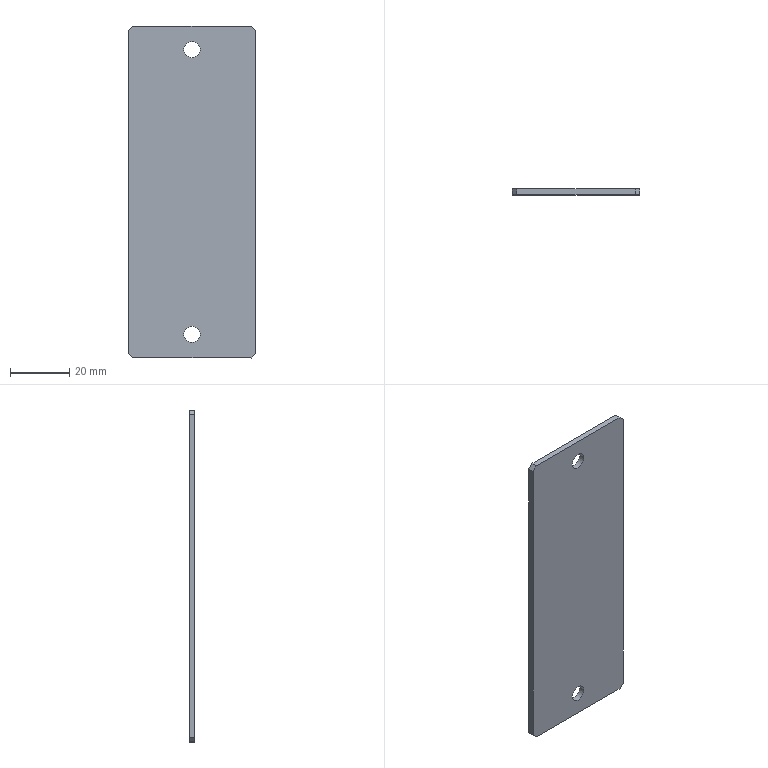Part | NX | 1 solid | 12 faces | box 43 x 2 x 112 mm | volume 9528 mm3 | plane 10 | cylinder 2 | commonest cylinder face diameters 5.5 x2
STEP:
#1=CARTESIAN_POINT('',(21.5,2.,54.5));
#2=VERTEX_POINT('',#1);
#3=CARTESIAN_POINT('',(21.5,2.,-54.5));
#4=VERTEX_POINT('',#3);
#5=CARTESIAN_POINT('',(21.5,2.,-56.));
#6=DIRECTION('',(0.,0.,-1.));
#7=VECTOR('',#6,1000.);
#8=LINE('',#5,#7);
#9=EDGE_CURVE('',#2,#4,#8,.T.);
#10=ORIENTED_EDGE('',*,*,#9,.F.);
#11=CARTESIAN_POINT('',(21.5,0.,54.5));
#12=VERTEX_POINT('',#11);
#13=CARTESIAN_POINT('',(21.5,2.,54.5));
#14=DIRECTION('',(0.,-1.,0.));
#15=VECTOR('',#14,1000.);
#16=LINE('',#13,#15);
#17=EDGE_CURVE('',#2,#12,#16,.T.);
#18=ORIENTED_EDGE('',*,*,#17,.T.);
#19=CARTESIAN_POINT('',(21.5,0.,-54.5));
#20=VERTEX_POINT('',#19);
#21=CARTESIAN_POINT('',(21.5,0.,-56.));
#22=DIRECTION('',(0.,0.,-1.));
#23=VECTOR('',#22,1000.);
#24=LINE('',#21,#23);
#25=EDGE_CURVE('',#12,#20,#24,.T.);
#26=ORIENTED_EDGE('',*,*,#25,.T.);
#27=CARTESIAN_POINT('',(21.5,2.,-54.5));
#28=DIRECTION('',(0.,1.,0.));
#29=VECTOR('',#28,1000.);
#30=LINE('',#27,#29);
#31=EDGE_CURVE('',#20,#4,#30,.T.);
#32=ORIENTED_EDGE('',*,*,#31,.T.);
#33=EDGE_LOOP('',(#10,#18,#26,#32));
#34=FACE_BOUND('',#33,.T.);
#35=CARTESIAN_POINT('',(21.5,2.,-56.));
#36=DIRECTION('',(-1.,0.,0.));
#37=DIRECTION('',(0.,0.,1.));
#38=AXIS2_PLACEMENT_3D('',#35,#36,#37);
#39=PLANE('',#38);
#40=ADVANCED_FACE('',(#34),#39,.F.);
#41=CARTESIAN_POINT('',(20.,2.,-56.));
#42=VERTEX_POINT('',#41);
#43=CARTESIAN_POINT('',(-20.,2.,-56.));
#44=VERTEX_POINT('',#43);
#45=CARTESIAN_POINT('',(-21.5,2.,-56.));
#46=DIRECTION('',(-1.,0.,0.));
#47=VECTOR('',#46,1000.);
#48=LINE('',#45,#47);
#49=EDGE_CURVE('',#42,#44,#48,.T.);
#50=ORIENTED_EDGE('',*,*,#49,.F.);
#51=CARTESIAN_POINT('',(20.,0.,-56.));
#52=VERTEX_POINT('',#51);
#53=CARTESIAN_POINT('',(20.,2.,-56.));
#54=DIRECTION('',(0.,-1.,0.));
#55=VECTOR('',#54,1000.);
#56=LINE('',#53,#55);
#57=EDGE_CURVE('',#42,#52,#56,.T.);
#58=ORIENTED_EDGE('',*,*,#57,.T.);
#59=CARTESIAN_POINT('',(-20.,0.,-56.));
#60=VERTEX_POINT('',#59);
#61=CARTESIAN_POINT('',(-21.5,0.,-56.));
#62=DIRECTION('',(-1.,0.,0.));
#63=VECTOR('',#62,1000.);
#64=LINE('',#61,#63);
#65=EDGE_CURVE('',#52,#60,#64,.T.);
#66=ORIENTED_EDGE('',*,*,#65,.T.);
#67=CARTESIAN_POINT('',(-20.,2.,-56.));
#68=DIRECTION('',(0.,1.,0.));
#69=VECTOR('',#68,1000.);
#70=LINE('',#67,#69);
#71=EDGE_CURVE('',#60,#44,#70,.T.);
#72=ORIENTED_EDGE('',*,*,#71,.T.);
#73=EDGE_LOOP('',(#50,#58,#66,#72));
#74=FACE_BOUND('',#73,.T.);
#75=CARTESIAN_POINT('',(-21.5,2.,-56.));
#76=DIRECTION('',(0.,0.,1.));
#77=DIRECTION('',(1.,0.,0.));
#78=AXIS2_PLACEMENT_3D('',#75,#76,#77);
#79=PLANE('',#78);
#80=ADVANCED_FACE('',(#74),#79,.F.);
#81=CARTESIAN_POINT('',(-21.5,0.,-54.5));
#82=VERTEX_POINT('',#81);
#83=CARTESIAN_POINT('',(-21.5,0.,54.5));
#84=VERTEX_POINT('',#83);
#85=CARTESIAN_POINT('',(-21.5,0.,-56.));
#86=DIRECTION('',(0.,0.,1.));
#87=VECTOR('',#86,1000.);
#88=LINE('',#85,#87);
#89=EDGE_CURVE('',#82,#84,#88,.T.);
#90=ORIENTED_EDGE('',*,*,#89,.T.);
#91=CARTESIAN_POINT('',(-21.5,2.,54.5));
#92=VERTEX_POINT('',#91);
#93=CARTESIAN_POINT('',(-21.5,2.,54.5));
#94=DIRECTION('',(0.,1.,0.));
#95=VECTOR('',#94,1000.);
#96=LINE('',#93,#95);
#97=EDGE_CURVE('',#84,#92,#96,.T.);
#98=ORIENTED_EDGE('',*,*,#97,.T.);
#99=CARTESIAN_POINT('',(-21.5,2.,-54.5));
#100=VERTEX_POINT('',#99);
#101=CARTESIAN_POINT('',(-21.5,2.,-56.));
#102=DIRECTION('',(0.,0.,1.));
#103=VECTOR('',#102,1000.);
#104=LINE('',#101,#103);
#105=EDGE_CURVE('',#100,#92,#104,.T.);
#106=ORIENTED_EDGE('',*,*,#105,.F.);
#107=CARTESIAN_POINT('',(-21.5,2.,-54.5));
#108=DIRECTION('',(0.,-1.,0.));
#109=VECTOR('',#108,1000.);
#110=LINE('',#107,#109);
#111=EDGE_CURVE('',#100,#82,#110,.T.);
#112=ORIENTED_EDGE('',*,*,#111,.T.);
#113=EDGE_LOOP('',(#90,#98,#106,#112));
#114=FACE_BOUND('',#113,.T.);
#115=CARTESIAN_POINT('',(-21.5,2.,-56.));
#116=DIRECTION('',(1.,0.,0.));
#117=DIRECTION('',(0.,0.,-1.));
#118=AXIS2_PLACEMENT_3D('',#115,#116,#117);
#119=PLANE('',#118);
#120=ADVANCED_FACE('',(#114),#119,.F.);
#121=CARTESIAN_POINT('',(-20.,2.,56.));
#122=VERTEX_POINT('',#121);
#123=CARTESIAN_POINT('',(20.,2.,56.));
#124=VERTEX_POINT('',#123);
#125=CARTESIAN_POINT('',(-21.5,2.,56.));
#126=DIRECTION('',(1.,0.,0.));
#127=VECTOR('',#126,1000.);
#128=LINE('',#125,#127);
#129=EDGE_CURVE('',#122,#124,#128,.T.);
#130=ORIENTED_EDGE('',*,*,#129,.F.);
#131=CARTESIAN_POINT('',(-20.,0.,56.));
#132=VERTEX_POINT('',#131);
#133=CARTESIAN_POINT('',(-20.,2.,56.));
#134=DIRECTION('',(0.,-1.,0.));
#135=VECTOR('',#134,1000.);
#136=LINE('',#133,#135);
#137=EDGE_CURVE('',#122,#132,#136,.T.);
#138=ORIENTED_EDGE('',*,*,#137,.T.);
#139=CARTESIAN_POINT('',(20.,0.,56.));
#140=VERTEX_POINT('',#139);
#141=CARTESIAN_POINT('',(-21.5,0.,56.));
#142=DIRECTION('',(1.,0.,0.));
#143=VECTOR('',#142,1000.);
#144=LINE('',#141,#143);
#145=EDGE_CURVE('',#132,#140,#144,.T.);
#146=ORIENTED_EDGE('',*,*,#145,.T.);
#147=CARTESIAN_POINT('',(20.,2.,56.));
#148=DIRECTION('',(0.,1.,0.));
#149=VECTOR('',#148,1000.);
#150=LINE('',#147,#149);
#151=EDGE_CURVE('',#140,#124,#150,.T.);
#152=ORIENTED_EDGE('',*,*,#151,.T.);
#153=EDGE_LOOP('',(#130,#138,#146,#152));
#154=FACE_BOUND('',#153,.T.);
#155=CARTESIAN_POINT('',(-21.5,2.,56.));
#156=DIRECTION('',(0.,0.,-1.));
#157=DIRECTION('',(-1.,0.,0.));
#158=AXIS2_PLACEMENT_3D('',#155,#156,#157);
#159=PLANE('',#158);
#160=ADVANCED_FACE('',(#154),#159,.F.);
#161=CARTESIAN_POINT('',(0.,2.,50.75));
#162=VERTEX_POINT('',#161);
#163=CARTESIAN_POINT('',(0.,2.,48.));
#164=DIRECTION('',(0.,1.,0.));
#165=DIRECTION('',(0.,0.,1.));
#166=AXIS2_PLACEMENT_3D('',#163,#164,#165);
#167=CIRCLE('',#166,2.75);
#168=EDGE_CURVE('',#162,#162,#167,.T.);
#169=ORIENTED_EDGE('',*,*,#168,.F.);
#170=EDGE_LOOP('',(#169));
#171=FACE_BOUND('',#170,.T.);
#172=CARTESIAN_POINT('',(0.,2.,-45.25));
#173=VERTEX_POINT('',#172);
#174=CARTESIAN_POINT('',(0.,2.,-48.));
#175=DIRECTION('',(0.,1.,0.));
#176=DIRECTION('',(0.,0.,1.));
#177=AXIS2_PLACEMENT_3D('',#174,#175,#176);
#178=CIRCLE('',#177,2.75);
#179=EDGE_CURVE('',#173,#173,#178,.T.);
#180=ORIENTED_EDGE('',*,*,#179,.F.);
#181=EDGE_LOOP('',(#180));
#182=FACE_BOUND('',#181,.T.);
#183=ORIENTED_EDGE('',*,*,#105,.T.);
#184=CARTESIAN_POINT('',(-38.,2.,38.));
#185=DIRECTION('',(-0.7071,0.,-0.7071));
#186=VECTOR('',#185,1000.);
#187=LINE('',#184,#186);
#188=EDGE_CURVE('',#92,#122,#187,.F.);
#189=ORIENTED_EDGE('',*,*,#188,.T.);
#190=ORIENTED_EDGE('',*,*,#129,.T.);
#191=CARTESIAN_POINT('',(38.,2.,38.));
#192=DIRECTION('',(-0.7071,0.,0.7071));
#193=VECTOR('',#192,1000.);
#194=LINE('',#191,#193);
#195=EDGE_CURVE('',#124,#2,#194,.F.);
#196=ORIENTED_EDGE('',*,*,#195,.T.);
#197=ORIENTED_EDGE('',*,*,#9,.T.);
#198=CARTESIAN_POINT('',(38.,2.,-38.));
#199=DIRECTION('',(0.7071,0.,0.7071));
#200=VECTOR('',#199,1000.);
#201=LINE('',#198,#200);
#202=EDGE_CURVE('',#4,#42,#201,.F.);
#203=ORIENTED_EDGE('',*,*,#202,.T.);
#204=ORIENTED_EDGE('',*,*,#49,.T.);
#205=CARTESIAN_POINT('',(-38.,2.,-38.));
#206=DIRECTION('',(0.7071,0.,-0.7071));
#207=VECTOR('',#206,1000.);
#208=LINE('',#205,#207);
#209=EDGE_CURVE('',#44,#100,#208,.F.);
#210=ORIENTED_EDGE('',*,*,#209,.T.);
#211=EDGE_LOOP('',(#183,#189,#190,#196,#197,#203,#204,#210));
#212=FACE_BOUND('',#211,.T.);
#213=CARTESIAN_POINT('',(0.,2.,0.));
#214=DIRECTION('',(0.,1.,0.));
#215=DIRECTION('',(0.,0.,1.));
#216=AXIS2_PLACEMENT_3D('',#213,#214,#215);
#217=PLANE('',#216);
#218=ADVANCED_FACE('',(#171,#182,#212),#217,.T.);
#219=CARTESIAN_POINT('',(0.,0.,50.75));
#220=VERTEX_POINT('',#219);
#221=CARTESIAN_POINT('',(0.,0.,48.));
#222=DIRECTION('',(0.,1.,0.));
#223=DIRECTION('',(0.,0.,1.));
#224=AXIS2_PLACEMENT_3D('',#221,#222,#223);
#225=CIRCLE('',#224,2.75);
#226=EDGE_CURVE('',#220,#220,#225,.T.);
#227=ORIENTED_EDGE('',*,*,#226,.T.);
#228=EDGE_LOOP('',(#227));
#229=FACE_BOUND('',#228,.T.);
#230=CARTESIAN_POINT('',(0.,0.,-45.25));
#231=VERTEX_POINT('',#230);
#232=CARTESIAN_POINT('',(0.,0.,-48.));
#233=DIRECTION('',(0.,1.,0.));
#234=DIRECTION('',(0.,0.,1.));
#235=AXIS2_PLACEMENT_3D('',#232,#233,#234);
#236=CIRCLE('',#235,2.75);
#237=EDGE_CURVE('',#231,#231,#236,.T.);
#238=ORIENTED_EDGE('',*,*,#237,.T.);
#239=EDGE_LOOP('',(#238));
#240=FACE_BOUND('',#239,.T.);
#241=ORIENTED_EDGE('',*,*,#145,.F.);
#242=CARTESIAN_POINT('',(-20.,0.,56.));
#243=DIRECTION('',(0.7071,0.,0.7071));
#244=VECTOR('',#243,1000.);
#245=LINE('',#242,#244);
#246=EDGE_CURVE('',#132,#84,#245,.F.);
#247=ORIENTED_EDGE('',*,*,#246,.T.);
#248=ORIENTED_EDGE('',*,*,#89,.F.);
#249=CARTESIAN_POINT('',(-21.5,0.,-54.5));
#250=DIRECTION('',(-0.7071,0.,0.7071));
#251=VECTOR('',#250,1000.);
#252=LINE('',#249,#251);
#253=EDGE_CURVE('',#82,#60,#252,.F.);
#254=ORIENTED_EDGE('',*,*,#253,.T.);
#255=ORIENTED_EDGE('',*,*,#65,.F.);
#256=CARTESIAN_POINT('',(20.,0.,-56.));
#257=DIRECTION('',(-0.7071,0.,-0.7071));
#258=VECTOR('',#257,1000.);
#259=LINE('',#256,#258);
#260=EDGE_CURVE('',#52,#20,#259,.F.);
#261=ORIENTED_EDGE('',*,*,#260,.T.);
#262=ORIENTED_EDGE('',*,*,#25,.F.);
#263=CARTESIAN_POINT('',(21.5,0.,54.5));
#264=DIRECTION('',(0.7071,0.,-0.7071));
#265=VECTOR('',#264,1000.);
#266=LINE('',#263,#265);
#267=EDGE_CURVE('',#12,#140,#266,.F.);
#268=ORIENTED_EDGE('',*,*,#267,.T.);
#269=EDGE_LOOP('',(#241,#247,#248,#254,#255,#261,#262,#268));
#270=FACE_BOUND('',#269,.T.);
#271=CARTESIAN_POINT('',(0.,0.,0.));
#272=DIRECTION('',(0.,1.,0.));
#273=DIRECTION('',(0.,0.,1.));
#274=AXIS2_PLACEMENT_3D('',#271,#272,#273);
#275=PLANE('',#274);
#276=ADVANCED_FACE('',(#229,#240,#270),#275,.F.);
#277=ORIENTED_EDGE('',*,*,#237,.F.);
#278=EDGE_LOOP('',(#277));
#279=FACE_BOUND('',#278,.T.);
#280=ORIENTED_EDGE('',*,*,#179,.T.);
#281=EDGE_LOOP('',(#280));
#282=FACE_BOUND('',#281,.T.);
#283=CARTESIAN_POINT('',(0.,2.,-48.));
#284=DIRECTION('',(0.,1.,0.));
#285=DIRECTION('',(0.,0.,1.));
#286=AXIS2_PLACEMENT_3D('',#283,#284,#285);
#287=CYLINDRICAL_SURFACE('',#286,2.75);
#288=ADVANCED_FACE('',(#279,#282),#287,.F.);
#289=ORIENTED_EDGE('',*,*,#226,.F.);
#290=EDGE_LOOP('',(#289));
#291=FACE_BOUND('',#290,.T.);
#292=ORIENTED_EDGE('',*,*,#168,.T.);
#293=EDGE_LOOP('',(#292));
#294=FACE_BOUND('',#293,.T.);
#295=CARTESIAN_POINT('',(0.,2.,48.));
#296=DIRECTION('',(0.,1.,0.));
#297=DIRECTION('',(0.,0.,1.));
#298=AXIS2_PLACEMENT_3D('',#295,#296,#297);
#299=CYLINDRICAL_SURFACE('',#298,2.75);
#300=ADVANCED_FACE('',(#291,#294),#299,.F.);
#301=ORIENTED_EDGE('',*,*,#188,.F.);
#302=ORIENTED_EDGE('',*,*,#97,.F.);
#303=ORIENTED_EDGE('',*,*,#246,.F.);
#304=ORIENTED_EDGE('',*,*,#137,.F.);
#305=EDGE_LOOP('',(#301,#302,#303,#304));
#306=FACE_BOUND('',#305,.T.);
#307=CARTESIAN_POINT('',(-20.,2.,56.));
#308=DIRECTION('',(0.7071,0.,-0.7071));
#309=DIRECTION('',(0.,-1.,0.));
#310=AXIS2_PLACEMENT_3D('',#307,#308,#309);
#311=PLANE('',#310);
#312=ADVANCED_FACE('',(#306),#311,.F.);
#313=ORIENTED_EDGE('',*,*,#195,.F.);
#314=ORIENTED_EDGE('',*,*,#151,.F.);
#315=ORIENTED_EDGE('',*,*,#267,.F.);
#316=ORIENTED_EDGE('',*,*,#17,.F.);
#317=EDGE_LOOP('',(#313,#314,#315,#316));
#318=FACE_BOUND('',#317,.T.);
#319=CARTESIAN_POINT('',(21.5,2.,54.5));
#320=DIRECTION('',(-0.7071,0.,-0.7071));
#321=DIRECTION('',(0.,-1.,0.));
#322=AXIS2_PLACEMENT_3D('',#319,#320,#321);
#323=PLANE('',#322);
#324=ADVANCED_FACE('',(#318),#323,.F.);
#325=ORIENTED_EDGE('',*,*,#202,.F.);
#326=ORIENTED_EDGE('',*,*,#31,.F.);
#327=ORIENTED_EDGE('',*,*,#260,.F.);
#328=ORIENTED_EDGE('',*,*,#57,.F.);
#329=EDGE_LOOP('',(#325,#326,#327,#328));
#330=FACE_BOUND('',#329,.T.);
#331=CARTESIAN_POINT('',(20.,2.,-56.));
#332=DIRECTION('',(-0.7071,0.,0.7071));
#333=DIRECTION('',(0.,-1.,0.));
#334=AXIS2_PLACEMENT_3D('',#331,#332,#333);
#335=PLANE('',#334);
#336=ADVANCED_FACE('',(#330),#335,.F.);
#337=ORIENTED_EDGE('',*,*,#209,.F.);
#338=ORIENTED_EDGE('',*,*,#71,.F.);
#339=ORIENTED_EDGE('',*,*,#253,.F.);
#340=ORIENTED_EDGE('',*,*,#111,.F.);
#341=EDGE_LOOP('',(#337,#338,#339,#340));
#342=FACE_BOUND('',#341,.T.);
#343=CARTESIAN_POINT('',(-21.5,2.,-54.5));
#344=DIRECTION('',(0.7071,0.,0.7071));
#345=DIRECTION('',(0.,-1.,0.));
#346=AXIS2_PLACEMENT_3D('',#343,#344,#345);
#347=PLANE('',#346);
#348=ADVANCED_FACE('',(#342),#347,.F.);
#349=CLOSED_SHELL('',(#40,#80,#120,#160,#218,#276,#288,#300,#312,#324,#336,#348));
#350=MANIFOLD_SOLID_BREP('',#349);
#351=(LENGTH_UNIT()NAMED_UNIT(*)SI_UNIT(.MILLI.,.METRE.));
#352=UNCERTAINTY_MEASURE_WITH_UNIT(LENGTH_MEASURE(0.00001),#351,'','');
#353=(NAMED_UNIT(*)PLANE_ANGLE_UNIT()SI_UNIT($,.RADIAN.));
#354=(NAMED_UNIT(*)SI_UNIT($,.STERADIAN.)SOLID_ANGLE_UNIT());
#355=(GEOMETRIC_REPRESENTATION_CONTEXT(3)GLOBAL_UNCERTAINTY_ASSIGNED_CONTEXT((#352))GLOBAL_UNIT_ASSIGNED_CONTEXT((#351,#353,#354))REPRESENTATION_CONTEXT('',''));
#356=ADVANCED_BREP_SHAPE_REPRESENTATION('',(#350),#355);